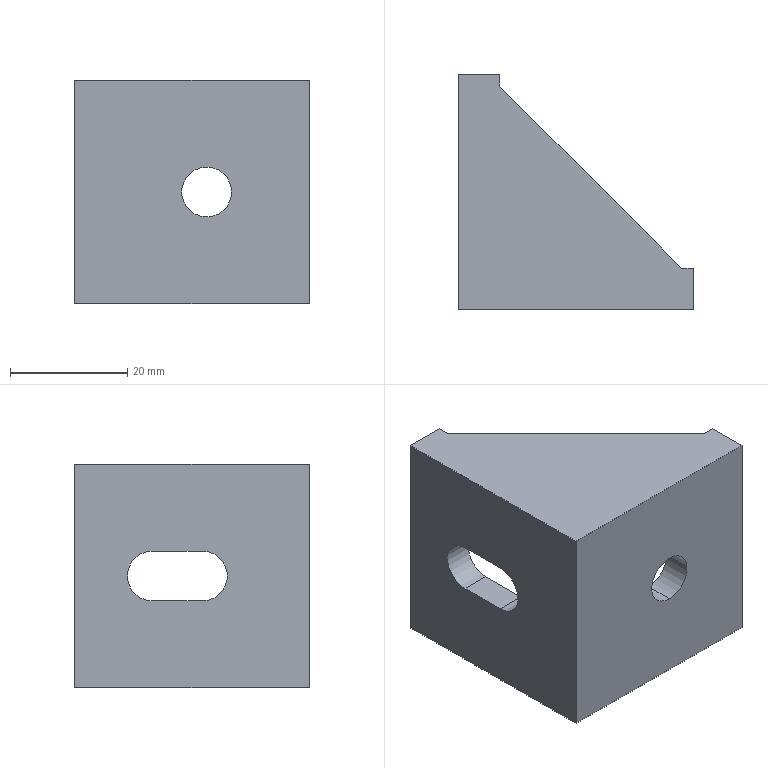Part | SolidWorks | features ICE 4, Extrusion 1 | 1 solid | 22 faces | box 40 x 40 x 38 mm | volume 15787 mm3 | plane 18 | cylinder 4 | commonest cylinder face diameters 8.5 x4
STEP:
#1=CARTESIAN_POINT('',(22.5,0.,14.75));
#2=VERTEX_POINT('',#1);
#3=CARTESIAN_POINT('',(22.5,0.,23.25));
#4=VERTEX_POINT('',#3);
#5=CARTESIAN_POINT('',(22.5,0.,19.));
#6=DIRECTION('',(0.,1.,0.));
#7=DIRECTION('',(0.,0.,1.));
#8=AXIS2_PLACEMENT_3D('',#5,#6,#7);
#9=CIRCLE('',#8,4.25);
#10=EDGE_CURVE('',#2,#4,#9,.T.);
#11=ORIENTED_EDGE('',*,*,#10,.F.);
#12=CARTESIAN_POINT('',(22.5,5.,14.75));
#13=VERTEX_POINT('',#12);
#14=CARTESIAN_POINT('',(22.5,0.,14.75));
#15=DIRECTION('',(0.,1.,0.));
#16=VECTOR('',#15,1000.);
#17=LINE('',#14,#16);
#18=EDGE_CURVE('',#2,#13,#17,.T.);
#19=ORIENTED_EDGE('',*,*,#18,.T.);
#20=CARTESIAN_POINT('',(22.5,5.,23.25));
#21=VERTEX_POINT('',#20);
#22=CARTESIAN_POINT('',(22.5,5.,19.));
#23=DIRECTION('',(0.,1.,0.));
#24=DIRECTION('',(0.,0.,1.));
#25=AXIS2_PLACEMENT_3D('',#22,#23,#24);
#26=CIRCLE('',#25,4.25);
#27=EDGE_CURVE('',#13,#21,#26,.T.);
#28=ORIENTED_EDGE('',*,*,#27,.T.);
#29=CARTESIAN_POINT('',(22.5,0.,23.25));
#30=DIRECTION('',(0.,1.,0.));
#31=VECTOR('',#30,1000.);
#32=LINE('',#29,#31);
#33=EDGE_CURVE('',#4,#21,#32,.T.);
#34=ORIENTED_EDGE('',*,*,#33,.F.);
#35=EDGE_LOOP('',(#11,#19,#28,#34));
#36=FACE_OUTER_BOUND('',#35,.T.);
#37=CARTESIAN_POINT('',(22.5,0.,19.));
#38=DIRECTION('',(0.,1.,0.));
#39=DIRECTION('',(0.,0.,1.));
#40=AXIS2_PLACEMENT_3D('',#37,#38,#39);
#41=CYLINDRICAL_SURFACE('',#40,4.25);
#42=ADVANCED_FACE('',(#36),#41,.F.);
#43=CARTESIAN_POINT('',(22.5,5.,19.));
#44=DIRECTION('',(0.,1.,0.));
#45=DIRECTION('',(0.,0.,1.));
#46=AXIS2_PLACEMENT_3D('',#43,#44,#45);
#47=CIRCLE('',#46,4.25);
#48=EDGE_CURVE('',#21,#13,#47,.T.);
#49=ORIENTED_EDGE('',*,*,#48,.F.);
#50=ORIENTED_EDGE('',*,*,#27,.F.);
#51=EDGE_LOOP('',(#49,#50));
#52=FACE_BOUND('',#51,.T.);
#53=CARTESIAN_POINT('',(40.,5.,2.));
#54=VERTEX_POINT('',#53);
#55=CARTESIAN_POINT('',(5.,5.,2.));
#56=VERTEX_POINT('',#55);
#57=CARTESIAN_POINT('',(5.,5.,2.));
#58=DIRECTION('',(-1.,0.,0.));
#59=VECTOR('',#58,1000.);
#60=LINE('',#57,#59);
#61=EDGE_CURVE('',#54,#56,#60,.T.);
#62=ORIENTED_EDGE('',*,*,#61,.T.);
#63=CARTESIAN_POINT('',(5.,5.,36.));
#64=VERTEX_POINT('',#63);
#65=CARTESIAN_POINT('',(5.,5.,38.));
#66=DIRECTION('',(0.,0.,-1.));
#67=VECTOR('',#66,1000.);
#68=LINE('',#65,#67);
#69=EDGE_CURVE('',#64,#56,#68,.T.);
#70=ORIENTED_EDGE('',*,*,#69,.F.);
#71=CARTESIAN_POINT('',(40.,5.,36.));
#72=VERTEX_POINT('',#71);
#73=CARTESIAN_POINT('',(40.,5.,36.));
#74=DIRECTION('',(1.,0.,0.));
#75=VECTOR('',#74,1000.);
#76=LINE('',#73,#75);
#77=EDGE_CURVE('',#64,#72,#76,.T.);
#78=ORIENTED_EDGE('',*,*,#77,.T.);
#79=CARTESIAN_POINT('',(40.,5.,38.));
#80=DIRECTION('',(0.,0.,-1.));
#81=VECTOR('',#80,1000.);
#82=LINE('',#79,#81);
#83=EDGE_CURVE('',#72,#54,#82,.T.);
#84=ORIENTED_EDGE('',*,*,#83,.T.);
#85=EDGE_LOOP('',(#62,#70,#78,#84));
#86=FACE_OUTER_BOUND('',#85,.T.);
#87=CARTESIAN_POINT('',(5.,5.,38.));
#88=DIRECTION('',(0.,-1.,0.));
#89=DIRECTION('',(0.,0.,-1.));
#90=AXIS2_PLACEMENT_3D('',#87,#88,#89);
#91=PLANE('',#90);
#92=ADVANCED_FACE('',(#52,#86),#91,.F.);
#93=CARTESIAN_POINT('',(5.,18.25,23.25));
#94=VERTEX_POINT('',#93);
#95=CARTESIAN_POINT('',(5.,26.75,23.25));
#96=VERTEX_POINT('',#95);
#97=CARTESIAN_POINT('',(5.,5.,23.25));
#98=DIRECTION('',(0.,1.,0.));
#99=VECTOR('',#98,1000.);
#100=LINE('',#97,#99);
#101=EDGE_CURVE('',#94,#96,#100,.T.);
#102=ORIENTED_EDGE('',*,*,#101,.T.);
#103=CARTESIAN_POINT('',(5.,26.75,14.75));
#104=VERTEX_POINT('',#103);
#105=CARTESIAN_POINT('',(5.,26.75,19.));
#106=DIRECTION('',(-1.,0.,0.));
#107=DIRECTION('',(0.,0.,1.));
#108=AXIS2_PLACEMENT_3D('',#105,#106,#107);
#109=CIRCLE('',#108,4.25);
#110=EDGE_CURVE('',#96,#104,#109,.T.);
#111=ORIENTED_EDGE('',*,*,#110,.T.);
#112=CARTESIAN_POINT('',(5.,18.25,14.75));
#113=VERTEX_POINT('',#112);
#114=CARTESIAN_POINT('',(5.,5.,14.75));
#115=DIRECTION('',(0.,-1.,0.));
#116=VECTOR('',#115,1000.);
#117=LINE('',#114,#116);
#118=EDGE_CURVE('',#104,#113,#117,.T.);
#119=ORIENTED_EDGE('',*,*,#118,.T.);
#120=CARTESIAN_POINT('',(5.,18.25,19.));
#121=DIRECTION('',(-1.,0.,0.));
#122=DIRECTION('',(0.,0.,1.));
#123=AXIS2_PLACEMENT_3D('',#120,#121,#122);
#124=CIRCLE('',#123,4.25);
#125=EDGE_CURVE('',#113,#94,#124,.T.);
#126=ORIENTED_EDGE('',*,*,#125,.T.);
#127=EDGE_LOOP('',(#102,#111,#119,#126));
#128=FACE_BOUND('',#127,.T.);
#129=CARTESIAN_POINT('',(5.,40.,2.));
#130=VERTEX_POINT('',#129);
#131=CARTESIAN_POINT('',(5.,5.,2.));
#132=DIRECTION('',(0.,1.,0.));
#133=VECTOR('',#132,1000.);
#134=LINE('',#131,#133);
#135=EDGE_CURVE('',#56,#130,#134,.T.);
#136=ORIENTED_EDGE('',*,*,#135,.T.);
#137=CARTESIAN_POINT('',(5.,40.,36.));
#138=VERTEX_POINT('',#137);
#139=CARTESIAN_POINT('',(5.,40.,38.));
#140=DIRECTION('',(0.,0.,-1.));
#141=VECTOR('',#140,1000.);
#142=LINE('',#139,#141);
#143=EDGE_CURVE('',#138,#130,#142,.T.);
#144=ORIENTED_EDGE('',*,*,#143,.F.);
#145=CARTESIAN_POINT('',(5.,5.,36.));
#146=DIRECTION('',(0.,-1.,0.));
#147=VECTOR('',#146,1000.);
#148=LINE('',#145,#147);
#149=EDGE_CURVE('',#138,#64,#148,.T.);
#150=ORIENTED_EDGE('',*,*,#149,.T.);
#151=ORIENTED_EDGE('',*,*,#69,.T.);
#152=EDGE_LOOP('',(#136,#144,#150,#151));
#153=FACE_OUTER_BOUND('',#152,.T.);
#154=CARTESIAN_POINT('',(5.,5.,38.));
#155=DIRECTION('',(-1.,0.,0.));
#156=DIRECTION('',(0.,0.,1.));
#157=AXIS2_PLACEMENT_3D('',#154,#155,#156);
#158=PLANE('',#157);
#159=ADVANCED_FACE('',(#128,#153),#158,.F.);
#160=CARTESIAN_POINT('',(0.,26.75,14.75));
#161=VERTEX_POINT('',#160);
#162=CARTESIAN_POINT('',(0.,18.25,14.75));
#163=VERTEX_POINT('',#162);
#164=CARTESIAN_POINT('',(0.,22.5,14.75));
#165=DIRECTION('',(0.,-1.,0.));
#166=VECTOR('',#165,1000.);
#167=LINE('',#164,#166);
#168=EDGE_CURVE('',#161,#163,#167,.T.);
#169=ORIENTED_EDGE('',*,*,#168,.F.);
#170=CARTESIAN_POINT('',(0.,26.75,23.25));
#171=VERTEX_POINT('',#170);
#172=CARTESIAN_POINT('',(0.,26.75,19.));
#173=DIRECTION('',(-1.,0.,0.));
#174=DIRECTION('',(0.,0.,1.));
#175=AXIS2_PLACEMENT_3D('',#172,#173,#174);
#176=CIRCLE('',#175,4.25);
#177=EDGE_CURVE('',#171,#161,#176,.T.);
#178=ORIENTED_EDGE('',*,*,#177,.F.);
#179=CARTESIAN_POINT('',(0.,18.25,23.25));
#180=VERTEX_POINT('',#179);
#181=CARTESIAN_POINT('',(0.,18.25,23.25));
#182=DIRECTION('',(0.,1.,0.));
#183=VECTOR('',#182,1000.);
#184=LINE('',#181,#183);
#185=EDGE_CURVE('',#180,#171,#184,.T.);
#186=ORIENTED_EDGE('',*,*,#185,.F.);
#187=CARTESIAN_POINT('',(0.,18.25,19.));
#188=DIRECTION('',(-1.,0.,0.));
#189=DIRECTION('',(0.,0.,1.));
#190=AXIS2_PLACEMENT_3D('',#187,#188,#189);
#191=CIRCLE('',#190,4.25);
#192=EDGE_CURVE('',#163,#180,#191,.T.);
#193=ORIENTED_EDGE('',*,*,#192,.F.);
#194=EDGE_LOOP('',(#169,#178,#186,#193));
#195=FACE_BOUND('',#194,.T.);
#196=CARTESIAN_POINT('',(0.,40.,0.));
#197=VERTEX_POINT('',#196);
#198=CARTESIAN_POINT('',(0.,0.,0.));
#199=VERTEX_POINT('',#198);
#200=CARTESIAN_POINT('',(0.,0.,0.));
#201=DIRECTION('',(0.,-1.,0.));
#202=VECTOR('',#201,1000.);
#203=LINE('',#200,#202);
#204=EDGE_CURVE('',#197,#199,#203,.T.);
#205=ORIENTED_EDGE('',*,*,#204,.T.);
#206=CARTESIAN_POINT('',(0.,0.,38.));
#207=VERTEX_POINT('',#206);
#208=CARTESIAN_POINT('',(0.,0.,38.));
#209=DIRECTION('',(0.,0.,-1.));
#210=VECTOR('',#209,1000.);
#211=LINE('',#208,#210);
#212=EDGE_CURVE('',#207,#199,#211,.T.);
#213=ORIENTED_EDGE('',*,*,#212,.F.);
#214=CARTESIAN_POINT('',(0.,40.,38.));
#215=VERTEX_POINT('',#214);
#216=CARTESIAN_POINT('',(0.,0.,38.));
#217=DIRECTION('',(0.,-1.,0.));
#218=VECTOR('',#217,1000.);
#219=LINE('',#216,#218);
#220=EDGE_CURVE('',#215,#207,#219,.T.);
#221=ORIENTED_EDGE('',*,*,#220,.F.);
#222=CARTESIAN_POINT('',(0.,40.,38.));
#223=DIRECTION('',(0.,0.,-1.));
#224=VECTOR('',#223,1000.);
#225=LINE('',#222,#224);
#226=EDGE_CURVE('',#215,#197,#225,.T.);
#227=ORIENTED_EDGE('',*,*,#226,.T.);
#228=EDGE_LOOP('',(#205,#213,#221,#227));
#229=FACE_OUTER_BOUND('',#228,.T.);
#230=CARTESIAN_POINT('',(0.,0.,38.));
#231=DIRECTION('',(1.,0.,0.));
#232=DIRECTION('',(0.,0.,-1.));
#233=AXIS2_PLACEMENT_3D('',#230,#231,#232);
#234=PLANE('',#233);
#235=ADVANCED_FACE('',(#195,#229),#234,.F.);
#236=CARTESIAN_POINT('',(22.5,0.,19.));
#237=DIRECTION('',(0.,1.,0.));
#238=DIRECTION('',(0.,0.,1.));
#239=AXIS2_PLACEMENT_3D('',#236,#237,#238);
#240=CIRCLE('',#239,4.25);
#241=EDGE_CURVE('',#4,#2,#240,.T.);
#242=ORIENTED_EDGE('',*,*,#241,.T.);
#243=ORIENTED_EDGE('',*,*,#10,.T.);
#244=EDGE_LOOP('',(#242,#243));
#245=FACE_BOUND('',#244,.T.);
#246=CARTESIAN_POINT('',(40.,0.,0.));
#247=VERTEX_POINT('',#246);
#248=CARTESIAN_POINT('',(0.,0.,0.));
#249=DIRECTION('',(1.,0.,0.));
#250=VECTOR('',#249,1000.);
#251=LINE('',#248,#250);
#252=EDGE_CURVE('',#199,#247,#251,.T.);
#253=ORIENTED_EDGE('',*,*,#252,.T.);
#254=CARTESIAN_POINT('',(40.,0.,38.));
#255=VERTEX_POINT('',#254);
#256=CARTESIAN_POINT('',(40.,0.,38.));
#257=DIRECTION('',(0.,0.,-1.));
#258=VECTOR('',#257,1000.);
#259=LINE('',#256,#258);
#260=EDGE_CURVE('',#255,#247,#259,.T.);
#261=ORIENTED_EDGE('',*,*,#260,.F.);
#262=CARTESIAN_POINT('',(0.,0.,38.));
#263=DIRECTION('',(1.,0.,0.));
#264=VECTOR('',#263,1000.);
#265=LINE('',#262,#264);
#266=EDGE_CURVE('',#207,#255,#265,.T.);
#267=ORIENTED_EDGE('',*,*,#266,.F.);
#268=ORIENTED_EDGE('',*,*,#212,.T.);
#269=EDGE_LOOP('',(#253,#261,#267,#268));
#270=FACE_OUTER_BOUND('',#269,.T.);
#271=CARTESIAN_POINT('',(0.,0.,38.));
#272=DIRECTION('',(0.,1.,0.));
#273=DIRECTION('',(0.,0.,1.));
#274=AXIS2_PLACEMENT_3D('',#271,#272,#273);
#275=PLANE('',#274);
#276=ADVANCED_FACE('',(#245,#270),#275,.F.);
#277=CARTESIAN_POINT('',(40.,7.,0.));
#278=VERTEX_POINT('',#277);
#279=CARTESIAN_POINT('',(40.,5.,0.));
#280=DIRECTION('',(0.,1.,0.));
#281=VECTOR('',#280,1000.);
#282=LINE('',#279,#281);
#283=EDGE_CURVE('',#247,#278,#282,.T.);
#284=ORIENTED_EDGE('',*,*,#283,.T.);
#285=CARTESIAN_POINT('',(40.,7.,2.));
#286=VERTEX_POINT('',#285);
#287=CARTESIAN_POINT('',(40.,7.,2.));
#288=DIRECTION('',(0.,0.,-1.));
#289=VECTOR('',#288,1000.);
#290=LINE('',#287,#289);
#291=EDGE_CURVE('',#286,#278,#290,.T.);
#292=ORIENTED_EDGE('',*,*,#291,.F.);
#293=CARTESIAN_POINT('',(40.,5.,2.));
#294=DIRECTION('',(0.,-1.,0.));
#295=VECTOR('',#294,1000.);
#296=LINE('',#293,#295);
#297=EDGE_CURVE('',#286,#54,#296,.T.);
#298=ORIENTED_EDGE('',*,*,#297,.T.);
#299=ORIENTED_EDGE('',*,*,#83,.F.);
#300=CARTESIAN_POINT('',(40.,7.,36.));
#301=VERTEX_POINT('',#300);
#302=CARTESIAN_POINT('',(40.,7.,36.));
#303=DIRECTION('',(0.,1.,0.));
#304=VECTOR('',#303,1000.);
#305=LINE('',#302,#304);
#306=EDGE_CURVE('',#72,#301,#305,.T.);
#307=ORIENTED_EDGE('',*,*,#306,.T.);
#308=CARTESIAN_POINT('',(40.,7.,38.));
#309=VERTEX_POINT('',#308);
#310=CARTESIAN_POINT('',(40.,7.,36.));
#311=DIRECTION('',(0.,0.,1.));
#312=VECTOR('',#311,1000.);
#313=LINE('',#310,#312);
#314=EDGE_CURVE('',#301,#309,#313,.T.);
#315=ORIENTED_EDGE('',*,*,#314,.T.);
#316=CARTESIAN_POINT('',(40.,5.,38.));
#317=DIRECTION('',(0.,1.,0.));
#318=VECTOR('',#317,1000.);
#319=LINE('',#316,#318);
#320=EDGE_CURVE('',#255,#309,#319,.T.);
#321=ORIENTED_EDGE('',*,*,#320,.F.);
#322=ORIENTED_EDGE('',*,*,#260,.T.);
#323=EDGE_LOOP('',(#284,#292,#298,#299,#307,#315,#321,#322));
#324=FACE_OUTER_BOUND('',#323,.T.);
#325=CARTESIAN_POINT('',(40.,5.,38.));
#326=DIRECTION('',(-1.,0.,0.));
#327=DIRECTION('',(0.,0.,1.));
#328=AXIS2_PLACEMENT_3D('',#325,#326,#327);
#329=PLANE('',#328);
#330=ADVANCED_FACE('',(#324),#329,.F.);
#331=CARTESIAN_POINT('',(7.,40.,0.));
#332=VERTEX_POINT('',#331);
#333=CARTESIAN_POINT('',(0.,40.,0.));
#334=DIRECTION('',(-1.,0.,0.));
#335=VECTOR('',#334,1000.);
#336=LINE('',#333,#335);
#337=EDGE_CURVE('',#332,#197,#336,.T.);
#338=ORIENTED_EDGE('',*,*,#337,.T.);
#339=ORIENTED_EDGE('',*,*,#226,.F.);
#340=CARTESIAN_POINT('',(7.,40.,38.));
#341=VERTEX_POINT('',#340);
#342=CARTESIAN_POINT('',(0.,40.,38.));
#343=DIRECTION('',(-1.,0.,0.));
#344=VECTOR('',#343,1000.);
#345=LINE('',#342,#344);
#346=EDGE_CURVE('',#341,#215,#345,.T.);
#347=ORIENTED_EDGE('',*,*,#346,.F.);
#348=CARTESIAN_POINT('',(7.,40.,36.));
#349=VERTEX_POINT('',#348);
#350=CARTESIAN_POINT('',(7.,40.,36.));
#351=DIRECTION('',(0.,0.,1.));
#352=VECTOR('',#351,1000.);
#353=LINE('',#350,#352);
#354=EDGE_CURVE('',#349,#341,#353,.T.);
#355=ORIENTED_EDGE('',*,*,#354,.F.);
#356=CARTESIAN_POINT('',(5.,40.,36.));
#357=DIRECTION('',(-1.,0.,0.));
#358=VECTOR('',#357,1000.);
#359=LINE('',#356,#358);
#360=EDGE_CURVE('',#349,#138,#359,.T.);
#361=ORIENTED_EDGE('',*,*,#360,.T.);
#362=ORIENTED_EDGE('',*,*,#143,.T.);
#363=CARTESIAN_POINT('',(7.,40.,2.));
#364=VERTEX_POINT('',#363);
#365=CARTESIAN_POINT('',(7.,40.,2.));
#366=DIRECTION('',(1.,0.,0.));
#367=VECTOR('',#366,1000.);
#368=LINE('',#365,#367);
#369=EDGE_CURVE('',#130,#364,#368,.T.);
#370=ORIENTED_EDGE('',*,*,#369,.T.);
#371=CARTESIAN_POINT('',(7.,40.,2.));
#372=DIRECTION('',(0.,0.,-1.));
#373=VECTOR('',#372,1000.);
#374=LINE('',#371,#373);
#375=EDGE_CURVE('',#364,#332,#374,.T.);
#376=ORIENTED_EDGE('',*,*,#375,.T.);
#377=EDGE_LOOP('',(#338,#339,#347,#355,#361,#362,#370,#376));
#378=FACE_OUTER_BOUND('',#377,.T.);
#379=CARTESIAN_POINT('',(0.,40.,38.));
#380=DIRECTION('',(0.,-1.,0.));
#381=DIRECTION('',(0.,0.,-1.));
#382=AXIS2_PLACEMENT_3D('',#379,#380,#381);
#383=PLANE('',#382);
#384=ADVANCED_FACE('',(#378),#383,.F.);
#385=ORIENTED_EDGE('',*,*,#220,.T.);
#386=ORIENTED_EDGE('',*,*,#266,.T.);
#387=ORIENTED_EDGE('',*,*,#320,.T.);
#388=CARTESIAN_POINT('',(38.,7.,38.));
#389=VERTEX_POINT('',#388);
#390=CARTESIAN_POINT('',(38.,7.,38.));
#391=DIRECTION('',(-1.,0.,0.));
#392=VECTOR('',#391,1000.);
#393=LINE('',#390,#392);
#394=EDGE_CURVE('',#309,#389,#393,.T.);
#395=ORIENTED_EDGE('',*,*,#394,.T.);
#396=CARTESIAN_POINT('',(7.,38.,38.));
#397=VERTEX_POINT('',#396);
#398=CARTESIAN_POINT('',(7.,38.,38.));
#399=DIRECTION('',(-0.7071,0.7071,0.));
#400=VECTOR('',#399,1000.);
#401=LINE('',#398,#400);
#402=EDGE_CURVE('',#389,#397,#401,.T.);
#403=ORIENTED_EDGE('',*,*,#402,.T.);
#404=CARTESIAN_POINT('',(7.,40.,38.));
#405=DIRECTION('',(0.,1.,0.));
#406=VECTOR('',#405,1000.);
#407=LINE('',#404,#406);
#408=EDGE_CURVE('',#397,#341,#407,.T.);
#409=ORIENTED_EDGE('',*,*,#408,.T.);
#410=ORIENTED_EDGE('',*,*,#346,.T.);
#411=EDGE_LOOP('',(#385,#386,#387,#395,#403,#409,#410));
#412=FACE_OUTER_BOUND('',#411,.T.);
#413=CARTESIAN_POINT('',(0.,0.,38.));
#414=DIRECTION('',(0.,0.,-1.));
#415=DIRECTION('',(-1.,0.,0.));
#416=AXIS2_PLACEMENT_3D('',#413,#414,#415);
#417=PLANE('',#416);
#418=ADVANCED_FACE('',(#412),#417,.F.);
#419=ORIENTED_EDGE('',*,*,#337,.F.);
#420=CARTESIAN_POINT('',(7.,38.,0.));
#421=VERTEX_POINT('',#420);
#422=CARTESIAN_POINT('',(7.,38.,0.));
#423=DIRECTION('',(0.,-1.,0.));
#424=VECTOR('',#423,1000.);
#425=LINE('',#422,#424);
#426=EDGE_CURVE('',#332,#421,#425,.T.);
#427=ORIENTED_EDGE('',*,*,#426,.T.);
#428=CARTESIAN_POINT('',(38.,7.,0.));
#429=VERTEX_POINT('',#428);
#430=CARTESIAN_POINT('',(38.,7.,0.));
#431=DIRECTION('',(0.7071,-0.7071,0.));
#432=VECTOR('',#431,1000.);
#433=LINE('',#430,#432);
#434=EDGE_CURVE('',#421,#429,#433,.T.);
#435=ORIENTED_EDGE('',*,*,#434,.T.);
#436=CARTESIAN_POINT('',(40.,7.,0.));
#437=DIRECTION('',(1.,0.,0.));
#438=VECTOR('',#437,1000.);
#439=LINE('',#436,#438);
#440=EDGE_CURVE('',#429,#278,#439,.T.);
#441=ORIENTED_EDGE('',*,*,#440,.T.);
#442=ORIENTED_EDGE('',*,*,#283,.F.);
#443=ORIENTED_EDGE('',*,*,#252,.F.);
#444=ORIENTED_EDGE('',*,*,#204,.F.);
#445=EDGE_LOOP('',(#419,#427,#435,#441,#442,#443,#444));
#446=FACE_OUTER_BOUND('',#445,.T.);
#447=CARTESIAN_POINT('',(0.,0.,0.));
#448=DIRECTION('',(0.,0.,-1.));
#449=DIRECTION('',(-1.,0.,0.));
#450=AXIS2_PLACEMENT_3D('',#447,#448,#449);
#451=PLANE('',#450);
#452=ADVANCED_FACE('',(#446),#451,.T.);
#453=ORIENTED_EDGE('',*,*,#394,.F.);
#454=ORIENTED_EDGE('',*,*,#314,.F.);
#455=CARTESIAN_POINT('',(38.,7.,36.));
#456=VERTEX_POINT('',#455);
#457=CARTESIAN_POINT('',(38.,7.,36.));
#458=DIRECTION('',(-1.,0.,0.));
#459=VECTOR('',#458,1000.);
#460=LINE('',#457,#459);
#461=EDGE_CURVE('',#301,#456,#460,.T.);
#462=ORIENTED_EDGE('',*,*,#461,.T.);
#463=CARTESIAN_POINT('',(38.,7.,36.));
#464=DIRECTION('',(0.,0.,1.));
#465=VECTOR('',#464,1000.);
#466=LINE('',#463,#465);
#467=EDGE_CURVE('',#456,#389,#466,.T.);
#468=ORIENTED_EDGE('',*,*,#467,.T.);
#469=EDGE_LOOP('',(#453,#454,#462,#468));
#470=FACE_OUTER_BOUND('',#469,.T.);
#471=CARTESIAN_POINT('',(38.,7.,36.));
#472=DIRECTION('',(0.,1.,0.));
#473=DIRECTION('',(0.,0.,1.));
#474=AXIS2_PLACEMENT_3D('',#471,#472,#473);
#475=PLANE('',#474);
#476=ADVANCED_FACE('',(#470),#475,.T.);
#477=ORIENTED_EDGE('',*,*,#408,.F.);
#478=CARTESIAN_POINT('',(7.,38.,36.));
#479=VERTEX_POINT('',#478);
#480=CARTESIAN_POINT('',(7.,38.,36.));
#481=DIRECTION('',(0.,0.,1.));
#482=VECTOR('',#481,1000.);
#483=LINE('',#480,#482);
#484=EDGE_CURVE('',#479,#397,#483,.T.);
#485=ORIENTED_EDGE('',*,*,#484,.F.);
#486=CARTESIAN_POINT('',(7.,40.,36.));
#487=DIRECTION('',(0.,1.,0.));
#488=VECTOR('',#487,1000.);
#489=LINE('',#486,#488);
#490=EDGE_CURVE('',#479,#349,#489,.T.);
#491=ORIENTED_EDGE('',*,*,#490,.T.);
#492=ORIENTED_EDGE('',*,*,#354,.T.);
#493=EDGE_LOOP('',(#477,#485,#491,#492));
#494=FACE_OUTER_BOUND('',#493,.T.);
#495=CARTESIAN_POINT('',(7.,40.,36.));
#496=DIRECTION('',(1.,0.,0.));
#497=DIRECTION('',(0.,0.,-1.));
#498=AXIS2_PLACEMENT_3D('',#495,#496,#497);
#499=PLANE('',#498);
#500=ADVANCED_FACE('',(#494),#499,.T.);
#501=ORIENTED_EDGE('',*,*,#402,.F.);
#502=ORIENTED_EDGE('',*,*,#467,.F.);
#503=CARTESIAN_POINT('',(7.,38.,36.));
#504=DIRECTION('',(-0.7071,0.7071,0.));
#505=VECTOR('',#504,1000.);
#506=LINE('',#503,#505);
#507=EDGE_CURVE('',#456,#479,#506,.T.);
#508=ORIENTED_EDGE('',*,*,#507,.T.);
#509=ORIENTED_EDGE('',*,*,#484,.T.);
#510=EDGE_LOOP('',(#501,#502,#508,#509));
#511=FACE_OUTER_BOUND('',#510,.T.);
#512=CARTESIAN_POINT('',(7.,38.,36.));
#513=DIRECTION('',(0.7071,0.7071,0.));
#514=DIRECTION('',(-0.7071,0.7071,0.));
#515=AXIS2_PLACEMENT_3D('',#512,#513,#514);
#516=PLANE('',#515);
#517=ADVANCED_FACE('',(#511),#516,.T.);
#518=ORIENTED_EDGE('',*,*,#461,.F.);
#519=ORIENTED_EDGE('',*,*,#306,.F.);
#520=ORIENTED_EDGE('',*,*,#77,.F.);
#521=ORIENTED_EDGE('',*,*,#149,.F.);
#522=ORIENTED_EDGE('',*,*,#360,.F.);
#523=ORIENTED_EDGE('',*,*,#490,.F.);
#524=ORIENTED_EDGE('',*,*,#507,.F.);
#525=EDGE_LOOP('',(#518,#519,#520,#521,#522,#523,#524));
#526=FACE_OUTER_BOUND('',#525,.T.);
#527=CARTESIAN_POINT('',(0.,0.,36.));
#528=DIRECTION('',(0.,0.,-1.));
#529=DIRECTION('',(-1.,0.,0.));
#530=AXIS2_PLACEMENT_3D('',#527,#528,#529);
#531=PLANE('',#530);
#532=ADVANCED_FACE('',(#526),#531,.T.);
#533=ORIENTED_EDGE('',*,*,#440,.F.);
#534=CARTESIAN_POINT('',(38.,7.,2.));
#535=VERTEX_POINT('',#534);
#536=CARTESIAN_POINT('',(38.,7.,2.));
#537=DIRECTION('',(0.,0.,-1.));
#538=VECTOR('',#537,1000.);
#539=LINE('',#536,#538);
#540=EDGE_CURVE('',#535,#429,#539,.T.);
#541=ORIENTED_EDGE('',*,*,#540,.F.);
#542=CARTESIAN_POINT('',(40.,7.,2.));
#543=DIRECTION('',(1.,0.,0.));
#544=VECTOR('',#543,1000.);
#545=LINE('',#542,#544);
#546=EDGE_CURVE('',#535,#286,#545,.T.);
#547=ORIENTED_EDGE('',*,*,#546,.T.);
#548=ORIENTED_EDGE('',*,*,#291,.T.);
#549=EDGE_LOOP('',(#533,#541,#547,#548));
#550=FACE_OUTER_BOUND('',#549,.T.);
#551=CARTESIAN_POINT('',(40.,7.,2.));
#552=DIRECTION('',(0.,1.,0.));
#553=DIRECTION('',(0.,0.,1.));
#554=AXIS2_PLACEMENT_3D('',#551,#552,#553);
#555=PLANE('',#554);
#556=ADVANCED_FACE('',(#550),#555,.T.);
#557=ORIENTED_EDGE('',*,*,#434,.F.);
#558=CARTESIAN_POINT('',(7.,38.,2.));
#559=VERTEX_POINT('',#558);
#560=CARTESIAN_POINT('',(7.,38.,2.));
#561=DIRECTION('',(0.,0.,-1.));
#562=VECTOR('',#561,1000.);
#563=LINE('',#560,#562);
#564=EDGE_CURVE('',#559,#421,#563,.T.);
#565=ORIENTED_EDGE('',*,*,#564,.F.);
#566=CARTESIAN_POINT('',(38.,7.,2.));
#567=DIRECTION('',(0.7071,-0.7071,0.));
#568=VECTOR('',#567,1000.);
#569=LINE('',#566,#568);
#570=EDGE_CURVE('',#559,#535,#569,.T.);
#571=ORIENTED_EDGE('',*,*,#570,.T.);
#572=ORIENTED_EDGE('',*,*,#540,.T.);
#573=EDGE_LOOP('',(#557,#565,#571,#572));
#574=FACE_OUTER_BOUND('',#573,.T.);
#575=CARTESIAN_POINT('',(38.,7.,2.));
#576=DIRECTION('',(0.7071,0.7071,0.));
#577=DIRECTION('',(-0.7071,0.7071,0.));
#578=AXIS2_PLACEMENT_3D('',#575,#576,#577);
#579=PLANE('',#578);
#580=ADVANCED_FACE('',(#574),#579,.T.);
#581=ORIENTED_EDGE('',*,*,#426,.F.);
#582=ORIENTED_EDGE('',*,*,#375,.F.);
#583=CARTESIAN_POINT('',(7.,38.,2.));
#584=DIRECTION('',(0.,-1.,0.));
#585=VECTOR('',#584,1000.);
#586=LINE('',#583,#585);
#587=EDGE_CURVE('',#364,#559,#586,.T.);
#588=ORIENTED_EDGE('',*,*,#587,.T.);
#589=ORIENTED_EDGE('',*,*,#564,.T.);
#590=EDGE_LOOP('',(#581,#582,#588,#589));
#591=FACE_OUTER_BOUND('',#590,.T.);
#592=CARTESIAN_POINT('',(7.,38.,2.));
#593=DIRECTION('',(1.,0.,0.));
#594=DIRECTION('',(0.,0.,-1.));
#595=AXIS2_PLACEMENT_3D('',#592,#593,#594);
#596=PLANE('',#595);
#597=ADVANCED_FACE('',(#591),#596,.T.);
#598=ORIENTED_EDGE('',*,*,#546,.F.);
#599=ORIENTED_EDGE('',*,*,#570,.F.);
#600=ORIENTED_EDGE('',*,*,#587,.F.);
#601=ORIENTED_EDGE('',*,*,#369,.F.);
#602=ORIENTED_EDGE('',*,*,#135,.F.);
#603=ORIENTED_EDGE('',*,*,#61,.F.);
#604=ORIENTED_EDGE('',*,*,#297,.F.);
#605=EDGE_LOOP('',(#598,#599,#600,#601,#602,#603,#604));
#606=FACE_OUTER_BOUND('',#605,.T.);
#607=CARTESIAN_POINT('',(0.,0.,2.));
#608=DIRECTION('',(0.,0.,-1.));
#609=DIRECTION('',(-1.,0.,0.));
#610=AXIS2_PLACEMENT_3D('',#607,#608,#609);
#611=PLANE('',#610);
#612=ADVANCED_FACE('',(#606),#611,.F.);
#613=ORIENTED_EDGE('',*,*,#18,.F.);
#614=ORIENTED_EDGE('',*,*,#241,.F.);
#615=ORIENTED_EDGE('',*,*,#33,.T.);
#616=ORIENTED_EDGE('',*,*,#48,.T.);
#617=EDGE_LOOP('',(#613,#614,#615,#616));
#618=FACE_OUTER_BOUND('',#617,.T.);
#619=CARTESIAN_POINT('',(22.5,0.,19.));
#620=DIRECTION('',(0.,1.,0.));
#621=DIRECTION('',(0.,0.,1.));
#622=AXIS2_PLACEMENT_3D('',#619,#620,#621);
#623=CYLINDRICAL_SURFACE('',#622,4.25);
#624=ADVANCED_FACE('',(#618),#623,.F.);
#625=CARTESIAN_POINT('',(40.,26.75,23.25));
#626=DIRECTION('',(-1.,0.,0.));
#627=VECTOR('',#626,1000.);
#628=LINE('',#625,#627);
#629=EDGE_CURVE('',#96,#171,#628,.T.);
#630=ORIENTED_EDGE('',*,*,#629,.T.);
#631=ORIENTED_EDGE('',*,*,#177,.T.);
#632=CARTESIAN_POINT('',(40.,26.75,14.75));
#633=DIRECTION('',(-1.,0.,0.));
#634=VECTOR('',#633,1000.);
#635=LINE('',#632,#634);
#636=EDGE_CURVE('',#104,#161,#635,.T.);
#637=ORIENTED_EDGE('',*,*,#636,.F.);
#638=ORIENTED_EDGE('',*,*,#110,.F.);
#639=EDGE_LOOP('',(#630,#631,#637,#638));
#640=FACE_OUTER_BOUND('',#639,.T.);
#641=CARTESIAN_POINT('',(40.,26.75,19.));
#642=DIRECTION('',(-1.,0.,0.));
#643=DIRECTION('',(0.,0.,1.));
#644=AXIS2_PLACEMENT_3D('',#641,#642,#643);
#645=CYLINDRICAL_SURFACE('',#644,4.25);
#646=ADVANCED_FACE('',(#640),#645,.F.);
#647=CARTESIAN_POINT('',(40.,18.25,23.25));
#648=DIRECTION('',(-1.,0.,0.));
#649=VECTOR('',#648,1000.);
#650=LINE('',#647,#649);
#651=EDGE_CURVE('',#94,#180,#650,.T.);
#652=ORIENTED_EDGE('',*,*,#651,.T.);
#653=ORIENTED_EDGE('',*,*,#185,.T.);
#654=ORIENTED_EDGE('',*,*,#629,.F.);
#655=ORIENTED_EDGE('',*,*,#101,.F.);
#656=EDGE_LOOP('',(#652,#653,#654,#655));
#657=FACE_OUTER_BOUND('',#656,.T.);
#658=CARTESIAN_POINT('',(40.,18.25,23.25));
#659=DIRECTION('',(0.,0.,1.));
#660=DIRECTION('',(0.,-1.,0.));
#661=AXIS2_PLACEMENT_3D('',#658,#659,#660);
#662=PLANE('',#661);
#663=ADVANCED_FACE('',(#657),#662,.F.);
#664=CARTESIAN_POINT('',(40.,18.25,14.75));
#665=DIRECTION('',(-1.,0.,0.));
#666=VECTOR('',#665,1000.);
#667=LINE('',#664,#666);
#668=EDGE_CURVE('',#113,#163,#667,.T.);
#669=ORIENTED_EDGE('',*,*,#668,.T.);
#670=ORIENTED_EDGE('',*,*,#192,.T.);
#671=ORIENTED_EDGE('',*,*,#651,.F.);
#672=ORIENTED_EDGE('',*,*,#125,.F.);
#673=EDGE_LOOP('',(#669,#670,#671,#672));
#674=FACE_OUTER_BOUND('',#673,.T.);
#675=CARTESIAN_POINT('',(40.,18.25,19.));
#676=DIRECTION('',(-1.,0.,0.));
#677=DIRECTION('',(0.,0.,1.));
#678=AXIS2_PLACEMENT_3D('',#675,#676,#677);
#679=CYLINDRICAL_SURFACE('',#678,4.25);
#680=ADVANCED_FACE('',(#674),#679,.F.);
#681=ORIENTED_EDGE('',*,*,#636,.T.);
#682=ORIENTED_EDGE('',*,*,#168,.T.);
#683=ORIENTED_EDGE('',*,*,#668,.F.);
#684=ORIENTED_EDGE('',*,*,#118,.F.);
#685=EDGE_LOOP('',(#681,#682,#683,#684));
#686=FACE_OUTER_BOUND('',#685,.T.);
#687=CARTESIAN_POINT('',(40.,22.5,14.75));
#688=DIRECTION('',(0.,0.,-1.));
#689=DIRECTION('',(-1.,0.,0.));
#690=AXIS2_PLACEMENT_3D('',#687,#688,#689);
#691=PLANE('',#690);
#692=ADVANCED_FACE('',(#686),#691,.F.);
#693=CLOSED_SHELL('',(#42,#92,#159,#235,#276,#330,#384,#418,#452,#476,#500,#517,#532,#556,#580,#597,#612,#624,#646,#663,#680,#692));
#694=MANIFOLD_SOLID_BREP('',#693);
#695=CARTESIAN_POINT('',(0.,0.,0.));
#696=DIRECTION('',(0.,0.,1.));
#697=DIRECTION('',(1.,0.,0.));
#698=AXIS2_PLACEMENT_3D('',#695,#696,#697);
#699=(LENGTH_UNIT()NAMED_UNIT(*)SI_UNIT(.MILLI.,.METRE.));
#700=UNCERTAINTY_MEASURE_WITH_UNIT(LENGTH_MEASURE(0.00001),#699,'','');
#701=(NAMED_UNIT(*)PLANE_ANGLE_UNIT()SI_UNIT($,.RADIAN.));
#702=(NAMED_UNIT(*)SI_UNIT($,.STERADIAN.)SOLID_ANGLE_UNIT());
#703=(GEOMETRIC_REPRESENTATION_CONTEXT(3)GLOBAL_UNCERTAINTY_ASSIGNED_CONTEXT((#700))GLOBAL_UNIT_ASSIGNED_CONTEXT((#699,#701,#702))REPRESENTATION_CONTEXT('',''));
#704=ADVANCED_BREP_SHAPE_REPRESENTATION('',(#694,#698),#703);